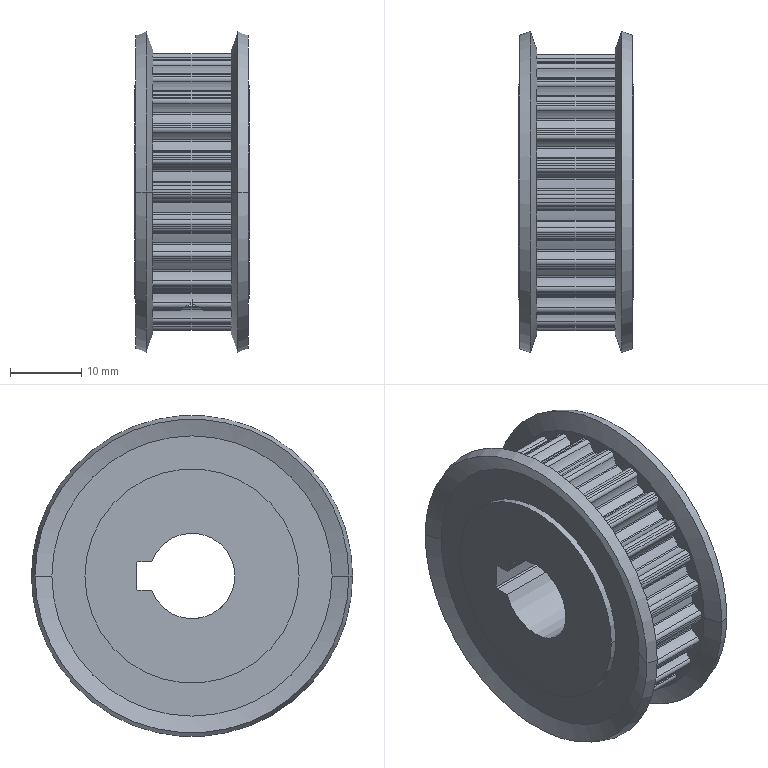Part | NX | 1 solid | 266 faces | box 16 x 45 x 45 mm | volume 15911 mm3 | cylinder 245 | cone 12 | plane 9 | commonest cylinder face diameters 0.5 x53 6.55 x53 1.1 x51 38.83 x51 35.29 x26 3.242 x4